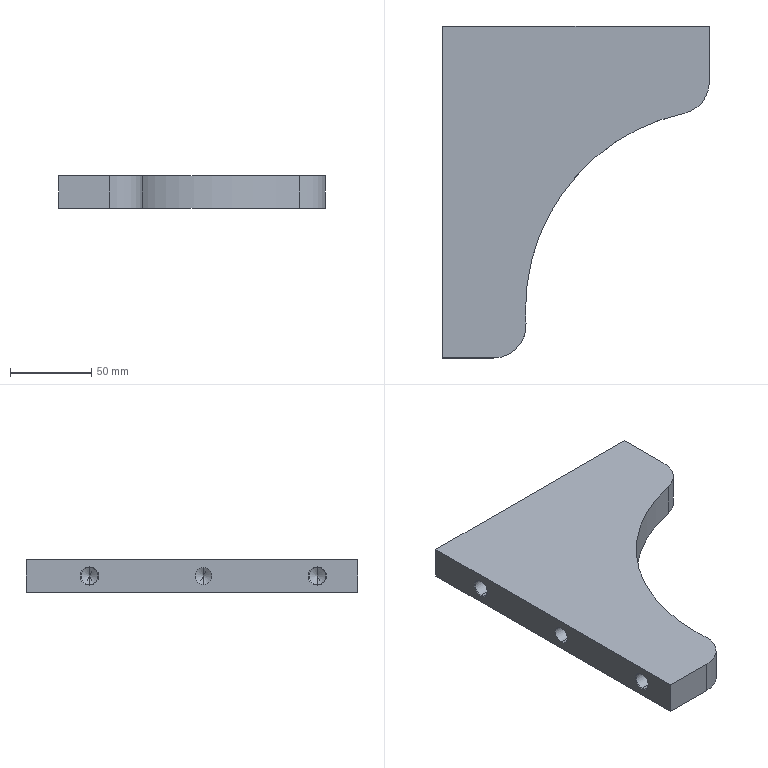Part | STEP file | 01-Driven chain press plate 2 | 1 solid | 26 faces | box 164 x 204 x 20 mm | volume 376718 mm3 | cone 10 | cylinder 10 | plane 6 | commonest cylinder face diameters 10.2 x6 40 x2 246 x2